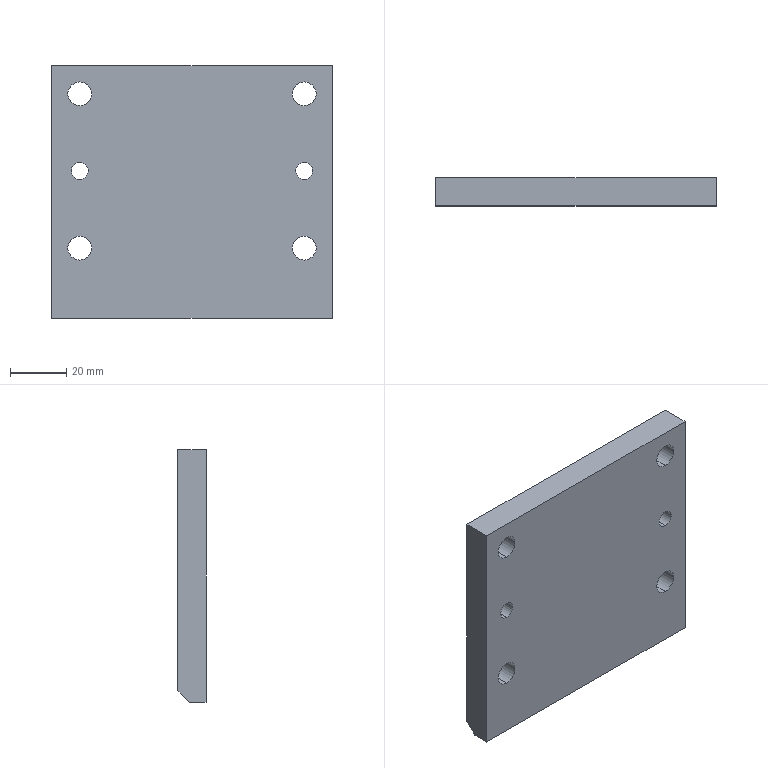Part | STEP file | X77-02101 | 1 solid | 19 faces | box 100 x 10 x 90 mm | volume 86365 mm3 | cylinder 12 | plane 7 | commonest cylinder face diameters 8.5 x8 6 x4
STEP:
#1=CARTESIAN_POINT('',(30.,-123.,55.5));
#2=VERTEX_POINT('',#1);
#3=CARTESIAN_POINT('',(30.,-123.,49.5));
#4=VERTEX_POINT('',#3);
#5=CARTESIAN_POINT('',(30.,-123.,52.5));
#6=DIRECTION('',(0.,-1.,0.));
#7=DIRECTION('',(0.,0.,1.));
#8=AXIS2_PLACEMENT_3D('',#5,#6,#7);
#9=CIRCLE('',#8,3.);
#10=EDGE_CURVE('',#2,#4,#9,.T.);
#11=ORIENTED_EDGE('',*,*,#10,.T.);
#12=CARTESIAN_POINT('',(30.,-113.,49.5));
#13=VERTEX_POINT('',#12);
#14=CARTESIAN_POINT('',(30.,-125.,49.5));
#15=DIRECTION('',(0.,1.,0.));
#16=VECTOR('',#15,1000.);
#17=LINE('',#14,#16);
#18=EDGE_CURVE('',#4,#13,#17,.T.);
#19=ORIENTED_EDGE('',*,*,#18,.T.);
#20=CARTESIAN_POINT('',(30.,-113.,55.5));
#21=VERTEX_POINT('',#20);
#22=CARTESIAN_POINT('',(30.,-113.,52.5));
#23=DIRECTION('',(0.,1.,0.));
#24=DIRECTION('',(0.,0.,1.));
#25=AXIS2_PLACEMENT_3D('',#22,#23,#24);
#26=CIRCLE('',#25,3.);
#27=EDGE_CURVE('',#13,#21,#26,.T.);
#28=ORIENTED_EDGE('',*,*,#27,.T.);
#29=CARTESIAN_POINT('',(30.,-125.,55.5));
#30=DIRECTION('',(0.,1.,0.));
#31=VECTOR('',#30,1000.);
#32=LINE('',#29,#31);
#33=EDGE_CURVE('',#2,#21,#32,.T.);
#34=ORIENTED_EDGE('',*,*,#33,.F.);
#35=EDGE_LOOP('',(#11,#19,#28,#34));
#36=FACE_OUTER_BOUND('',#35,.T.);
#37=CARTESIAN_POINT('',(30.,-125.,52.5));
#38=DIRECTION('',(0.,1.,0.));
#39=DIRECTION('',(0.,0.,1.));
#40=AXIS2_PLACEMENT_3D('',#37,#38,#39);
#41=CYLINDRICAL_SURFACE('',#40,3.);
#42=ADVANCED_FACE('',(#36),#41,.F.);
#43=CARTESIAN_POINT('',(-50.,-123.,55.5));
#44=VERTEX_POINT('',#43);
#45=CARTESIAN_POINT('',(-50.,-123.,49.5));
#46=VERTEX_POINT('',#45);
#47=CARTESIAN_POINT('',(-50.,-123.,52.5));
#48=DIRECTION('',(0.,-1.,0.));
#49=DIRECTION('',(0.,0.,1.));
#50=AXIS2_PLACEMENT_3D('',#47,#48,#49);
#51=CIRCLE('',#50,3.);
#52=EDGE_CURVE('',#44,#46,#51,.T.);
#53=ORIENTED_EDGE('',*,*,#52,.T.);
#54=CARTESIAN_POINT('',(-50.,-113.,49.5));
#55=VERTEX_POINT('',#54);
#56=CARTESIAN_POINT('',(-50.,-125.,49.5));
#57=DIRECTION('',(0.,1.,0.));
#58=VECTOR('',#57,1000.);
#59=LINE('',#56,#58);
#60=EDGE_CURVE('',#46,#55,#59,.T.);
#61=ORIENTED_EDGE('',*,*,#60,.T.);
#62=CARTESIAN_POINT('',(-50.,-113.,55.5));
#63=VERTEX_POINT('',#62);
#64=CARTESIAN_POINT('',(-50.,-113.,52.5));
#65=DIRECTION('',(0.,1.,0.));
#66=DIRECTION('',(0.,0.,1.));
#67=AXIS2_PLACEMENT_3D('',#64,#65,#66);
#68=CIRCLE('',#67,3.);
#69=EDGE_CURVE('',#55,#63,#68,.T.);
#70=ORIENTED_EDGE('',*,*,#69,.T.);
#71=CARTESIAN_POINT('',(-50.,-125.,55.5));
#72=DIRECTION('',(0.,1.,0.));
#73=VECTOR('',#72,1000.);
#74=LINE('',#71,#73);
#75=EDGE_CURVE('',#44,#63,#74,.T.);
#76=ORIENTED_EDGE('',*,*,#75,.F.);
#77=EDGE_LOOP('',(#53,#61,#70,#76));
#78=FACE_OUTER_BOUND('',#77,.T.);
#79=CARTESIAN_POINT('',(-50.,-125.,52.5));
#80=DIRECTION('',(0.,1.,0.));
#81=DIRECTION('',(0.,0.,1.));
#82=AXIS2_PLACEMENT_3D('',#79,#80,#81);
#83=CYLINDRICAL_SURFACE('',#82,3.);
#84=ADVANCED_FACE('',(#78),#83,.F.);
#85=CARTESIAN_POINT('',(-50.,-123.,84.25));
#86=VERTEX_POINT('',#85);
#87=CARTESIAN_POINT('',(-50.,-123.,75.75));
#88=VERTEX_POINT('',#87);
#89=CARTESIAN_POINT('',(-50.,-123.,80.));
#90=DIRECTION('',(0.,-1.,0.));
#91=DIRECTION('',(0.,0.,1.));
#92=AXIS2_PLACEMENT_3D('',#89,#90,#91);
#93=CIRCLE('',#92,4.25);
#94=EDGE_CURVE('',#86,#88,#93,.T.);
#95=ORIENTED_EDGE('',*,*,#94,.T.);
#96=CARTESIAN_POINT('',(-50.,-113.,75.75));
#97=VERTEX_POINT('',#96);
#98=CARTESIAN_POINT('',(-50.,-113.,75.75));
#99=DIRECTION('',(0.,1.,0.));
#100=VECTOR('',#99,1000.);
#101=LINE('',#98,#100);
#102=EDGE_CURVE('',#88,#97,#101,.T.);
#103=ORIENTED_EDGE('',*,*,#102,.T.);
#104=CARTESIAN_POINT('',(-50.,-113.,84.25));
#105=VERTEX_POINT('',#104);
#106=CARTESIAN_POINT('',(-50.,-113.,80.));
#107=DIRECTION('',(0.,1.,0.));
#108=DIRECTION('',(0.,0.,1.));
#109=AXIS2_PLACEMENT_3D('',#106,#107,#108);
#110=CIRCLE('',#109,4.25);
#111=EDGE_CURVE('',#97,#105,#110,.T.);
#112=ORIENTED_EDGE('',*,*,#111,.T.);
#113=CARTESIAN_POINT('',(-50.,-113.,84.25));
#114=DIRECTION('',(0.,1.,0.));
#115=VECTOR('',#114,1000.);
#116=LINE('',#113,#115);
#117=EDGE_CURVE('',#86,#105,#116,.T.);
#118=ORIENTED_EDGE('',*,*,#117,.F.);
#119=EDGE_LOOP('',(#95,#103,#112,#118));
#120=FACE_OUTER_BOUND('',#119,.T.);
#121=CARTESIAN_POINT('',(-50.,-113.,80.));
#122=DIRECTION('',(0.,1.,0.));
#123=DIRECTION('',(0.,0.,1.));
#124=AXIS2_PLACEMENT_3D('',#121,#122,#123);
#125=CYLINDRICAL_SURFACE('',#124,4.25);
#126=ADVANCED_FACE('',(#120),#125,.F.);
#127=CARTESIAN_POINT('',(-50.,-123.,29.25));
#128=VERTEX_POINT('',#127);
#129=CARTESIAN_POINT('',(-50.,-123.,20.75));
#130=VERTEX_POINT('',#129);
#131=CARTESIAN_POINT('',(-50.,-123.,25.));
#132=DIRECTION('',(0.,-1.,0.));
#133=DIRECTION('',(0.,0.,1.));
#134=AXIS2_PLACEMENT_3D('',#131,#132,#133);
#135=CIRCLE('',#134,4.25);
#136=EDGE_CURVE('',#128,#130,#135,.T.);
#137=ORIENTED_EDGE('',*,*,#136,.T.);
#138=CARTESIAN_POINT('',(-50.,-113.,20.75));
#139=VERTEX_POINT('',#138);
#140=CARTESIAN_POINT('',(-50.,-113.,20.75));
#141=DIRECTION('',(0.,1.,0.));
#142=VECTOR('',#141,1000.);
#143=LINE('',#140,#142);
#144=EDGE_CURVE('',#130,#139,#143,.T.);
#145=ORIENTED_EDGE('',*,*,#144,.T.);
#146=CARTESIAN_POINT('',(-50.,-113.,29.25));
#147=VERTEX_POINT('',#146);
#148=CARTESIAN_POINT('',(-50.,-113.,25.));
#149=DIRECTION('',(0.,1.,0.));
#150=DIRECTION('',(0.,0.,1.));
#151=AXIS2_PLACEMENT_3D('',#148,#149,#150);
#152=CIRCLE('',#151,4.25);
#153=EDGE_CURVE('',#139,#147,#152,.T.);
#154=ORIENTED_EDGE('',*,*,#153,.T.);
#155=CARTESIAN_POINT('',(-50.,-113.,29.25));
#156=DIRECTION('',(0.,1.,0.));
#157=VECTOR('',#156,1000.);
#158=LINE('',#155,#157);
#159=EDGE_CURVE('',#128,#147,#158,.T.);
#160=ORIENTED_EDGE('',*,*,#159,.F.);
#161=EDGE_LOOP('',(#137,#145,#154,#160));
#162=FACE_OUTER_BOUND('',#161,.T.);
#163=CARTESIAN_POINT('',(-50.,-113.,25.));
#164=DIRECTION('',(0.,1.,0.));
#165=DIRECTION('',(0.,0.,1.));
#166=AXIS2_PLACEMENT_3D('',#163,#164,#165);
#167=CYLINDRICAL_SURFACE('',#166,4.25);
#168=ADVANCED_FACE('',(#162),#167,.F.);
#169=CARTESIAN_POINT('',(30.,-123.,29.25));
#170=VERTEX_POINT('',#169);
#171=CARTESIAN_POINT('',(30.,-123.,20.75));
#172=VERTEX_POINT('',#171);
#173=CARTESIAN_POINT('',(30.,-123.,25.));
#174=DIRECTION('',(0.,-1.,0.));
#175=DIRECTION('',(0.,0.,1.));
#176=AXIS2_PLACEMENT_3D('',#173,#174,#175);
#177=CIRCLE('',#176,4.25);
#178=EDGE_CURVE('',#170,#172,#177,.T.);
#179=ORIENTED_EDGE('',*,*,#178,.T.);
#180=CARTESIAN_POINT('',(30.,-113.,20.75));
#181=VERTEX_POINT('',#180);
#182=CARTESIAN_POINT('',(30.,-113.,20.75));
#183=DIRECTION('',(0.,1.,0.));
#184=VECTOR('',#183,1000.);
#185=LINE('',#182,#184);
#186=EDGE_CURVE('',#172,#181,#185,.T.);
#187=ORIENTED_EDGE('',*,*,#186,.T.);
#188=CARTESIAN_POINT('',(30.,-113.,29.25));
#189=VERTEX_POINT('',#188);
#190=CARTESIAN_POINT('',(30.,-113.,25.));
#191=DIRECTION('',(0.,1.,0.));
#192=DIRECTION('',(0.,0.,1.));
#193=AXIS2_PLACEMENT_3D('',#190,#191,#192);
#194=CIRCLE('',#193,4.25);
#195=EDGE_CURVE('',#181,#189,#194,.T.);
#196=ORIENTED_EDGE('',*,*,#195,.T.);
#197=CARTESIAN_POINT('',(30.,-113.,29.25));
#198=DIRECTION('',(0.,1.,0.));
#199=VECTOR('',#198,1000.);
#200=LINE('',#197,#199);
#201=EDGE_CURVE('',#170,#189,#200,.T.);
#202=ORIENTED_EDGE('',*,*,#201,.F.);
#203=EDGE_LOOP('',(#179,#187,#196,#202));
#204=FACE_OUTER_BOUND('',#203,.T.);
#205=CARTESIAN_POINT('',(30.,-113.,25.));
#206=DIRECTION('',(0.,1.,0.));
#207=DIRECTION('',(0.,0.,1.));
#208=AXIS2_PLACEMENT_3D('',#205,#206,#207);
#209=CYLINDRICAL_SURFACE('',#208,4.25);
#210=ADVANCED_FACE('',(#204),#209,.F.);
#211=CARTESIAN_POINT('',(30.,-123.,84.25));
#212=VERTEX_POINT('',#211);
#213=CARTESIAN_POINT('',(30.,-123.,75.75));
#214=VERTEX_POINT('',#213);
#215=CARTESIAN_POINT('',(30.,-123.,80.));
#216=DIRECTION('',(0.,-1.,0.));
#217=DIRECTION('',(0.,0.,1.));
#218=AXIS2_PLACEMENT_3D('',#215,#216,#217);
#219=CIRCLE('',#218,4.25);
#220=EDGE_CURVE('',#212,#214,#219,.T.);
#221=ORIENTED_EDGE('',*,*,#220,.T.);
#222=CARTESIAN_POINT('',(30.,-113.,75.75));
#223=VERTEX_POINT('',#222);
#224=CARTESIAN_POINT('',(30.,-113.,75.75));
#225=DIRECTION('',(0.,1.,0.));
#226=VECTOR('',#225,1000.);
#227=LINE('',#224,#226);
#228=EDGE_CURVE('',#214,#223,#227,.T.);
#229=ORIENTED_EDGE('',*,*,#228,.T.);
#230=CARTESIAN_POINT('',(30.,-113.,84.25));
#231=VERTEX_POINT('',#230);
#232=CARTESIAN_POINT('',(30.,-113.,80.));
#233=DIRECTION('',(0.,1.,0.));
#234=DIRECTION('',(0.,0.,1.));
#235=AXIS2_PLACEMENT_3D('',#232,#233,#234);
#236=CIRCLE('',#235,4.25);
#237=EDGE_CURVE('',#223,#231,#236,.T.);
#238=ORIENTED_EDGE('',*,*,#237,.T.);
#239=CARTESIAN_POINT('',(30.,-113.,84.25));
#240=DIRECTION('',(0.,1.,0.));
#241=VECTOR('',#240,1000.);
#242=LINE('',#239,#241);
#243=EDGE_CURVE('',#212,#231,#242,.T.);
#244=ORIENTED_EDGE('',*,*,#243,.F.);
#245=EDGE_LOOP('',(#221,#229,#238,#244));
#246=FACE_OUTER_BOUND('',#245,.T.);
#247=CARTESIAN_POINT('',(30.,-113.,80.));
#248=DIRECTION('',(0.,1.,0.));
#249=DIRECTION('',(0.,0.,1.));
#250=AXIS2_PLACEMENT_3D('',#247,#248,#249);
#251=CYLINDRICAL_SURFACE('',#250,4.25);
#252=ADVANCED_FACE('',(#246),#251,.F.);
#253=CARTESIAN_POINT('',(-60.,-117.,0.));
#254=VERTEX_POINT('',#253);
#255=CARTESIAN_POINT('',(-60.,-123.,0.));
#256=VERTEX_POINT('',#255);
#257=CARTESIAN_POINT('',(-60.,-125.,0.));
#258=DIRECTION('',(0.,-1.,0.));
#259=VECTOR('',#258,1000.);
#260=LINE('',#257,#259);
#261=EDGE_CURVE('',#254,#256,#260,.T.);
#262=ORIENTED_EDGE('',*,*,#261,.T.);
#263=CARTESIAN_POINT('',(-60.,-123.,90.));
#264=VERTEX_POINT('',#263);
#265=CARTESIAN_POINT('',(-60.,-123.,0.));
#266=DIRECTION('',(0.,0.,-1.));
#267=VECTOR('',#266,1000.);
#268=LINE('',#265,#267);
#269=EDGE_CURVE('',#264,#256,#268,.T.);
#270=ORIENTED_EDGE('',*,*,#269,.F.);
#271=CARTESIAN_POINT('',(-60.,-113.,90.));
#272=VERTEX_POINT('',#271);
#273=CARTESIAN_POINT('',(-60.,-125.,90.));
#274=DIRECTION('',(0.,-1.,0.));
#275=VECTOR('',#274,1000.);
#276=LINE('',#273,#275);
#277=EDGE_CURVE('',#272,#264,#276,.T.);
#278=ORIENTED_EDGE('',*,*,#277,.F.);
#279=CARTESIAN_POINT('',(-60.,-113.,4.));
#280=VERTEX_POINT('',#279);
#281=CARTESIAN_POINT('',(-60.,-113.,90.));
#282=DIRECTION('',(0.,0.,-1.));
#283=VECTOR('',#282,1000.);
#284=LINE('',#281,#283);
#285=EDGE_CURVE('',#272,#280,#284,.T.);
#286=ORIENTED_EDGE('',*,*,#285,.T.);
#287=CARTESIAN_POINT('',(-60.,-113.,4.));
#288=DIRECTION('',(0.,-0.7071,-0.7071));
#289=VECTOR('',#288,1000.);
#290=LINE('',#287,#289);
#291=EDGE_CURVE('',#280,#254,#290,.T.);
#292=ORIENTED_EDGE('',*,*,#291,.T.);
#293=EDGE_LOOP('',(#262,#270,#278,#286,#292));
#294=FACE_OUTER_BOUND('',#293,.T.);
#295=CARTESIAN_POINT('',(-60.,-125.,90.));
#296=DIRECTION('',(1.,0.,0.));
#297=DIRECTION('',(0.,0.,-1.));
#298=AXIS2_PLACEMENT_3D('',#295,#296,#297);
#299=PLANE('',#298);
#300=ADVANCED_FACE('',(#294),#299,.F.);
#301=CARTESIAN_POINT('',(40.,-123.,90.));
#302=VERTEX_POINT('',#301);
#303=CARTESIAN_POINT('',(40.,-113.,90.));
#304=VERTEX_POINT('',#303);
#305=CARTESIAN_POINT('',(40.,-125.,90.));
#306=DIRECTION('',(0.,1.,0.));
#307=VECTOR('',#306,1000.);
#308=LINE('',#305,#307);
#309=EDGE_CURVE('',#302,#304,#308,.T.);
#310=ORIENTED_EDGE('',*,*,#309,.F.);
#311=CARTESIAN_POINT('',(40.,-123.,0.));
#312=VERTEX_POINT('',#311);
#313=CARTESIAN_POINT('',(40.,-123.,0.));
#314=DIRECTION('',(0.,0.,-1.));
#315=VECTOR('',#314,1000.);
#316=LINE('',#313,#315);
#317=EDGE_CURVE('',#302,#312,#316,.T.);
#318=ORIENTED_EDGE('',*,*,#317,.T.);
#319=CARTESIAN_POINT('',(40.,-117.,0.));
#320=VERTEX_POINT('',#319);
#321=CARTESIAN_POINT('',(40.,-125.,0.));
#322=DIRECTION('',(0.,1.,0.));
#323=VECTOR('',#322,1000.);
#324=LINE('',#321,#323);
#325=EDGE_CURVE('',#312,#320,#324,.T.);
#326=ORIENTED_EDGE('',*,*,#325,.T.);
#327=CARTESIAN_POINT('',(40.,-113.,4.));
#328=VERTEX_POINT('',#327);
#329=CARTESIAN_POINT('',(40.,-113.,4.));
#330=DIRECTION('',(0.,0.7071,0.7071));
#331=VECTOR('',#330,1000.);
#332=LINE('',#329,#331);
#333=EDGE_CURVE('',#320,#328,#332,.T.);
#334=ORIENTED_EDGE('',*,*,#333,.T.);
#335=CARTESIAN_POINT('',(40.,-113.,90.));
#336=DIRECTION('',(0.,0.,-1.));
#337=VECTOR('',#336,1000.);
#338=LINE('',#335,#337);
#339=EDGE_CURVE('',#304,#328,#338,.T.);
#340=ORIENTED_EDGE('',*,*,#339,.F.);
#341=EDGE_LOOP('',(#310,#318,#326,#334,#340));
#342=FACE_OUTER_BOUND('',#341,.T.);
#343=CARTESIAN_POINT('',(40.,-125.,90.));
#344=DIRECTION('',(-1.,0.,0.));
#345=DIRECTION('',(0.,0.,1.));
#346=AXIS2_PLACEMENT_3D('',#343,#344,#345);
#347=PLANE('',#346);
#348=ADVANCED_FACE('',(#342),#347,.F.);
#349=CARTESIAN_POINT('',(30.,-113.,52.5));
#350=DIRECTION('',(0.,1.,0.));
#351=DIRECTION('',(0.,0.,1.));
#352=AXIS2_PLACEMENT_3D('',#349,#350,#351);
#353=CIRCLE('',#352,3.);
#354=EDGE_CURVE('',#21,#13,#353,.T.);
#355=ORIENTED_EDGE('',*,*,#354,.F.);
#356=ORIENTED_EDGE('',*,*,#27,.F.);
#357=EDGE_LOOP('',(#355,#356));
#358=FACE_BOUND('',#357,.T.);
#359=CARTESIAN_POINT('',(-50.,-113.,52.5));
#360=DIRECTION('',(0.,1.,0.));
#361=DIRECTION('',(0.,0.,1.));
#362=AXIS2_PLACEMENT_3D('',#359,#360,#361);
#363=CIRCLE('',#362,3.);
#364=EDGE_CURVE('',#63,#55,#363,.T.);
#365=ORIENTED_EDGE('',*,*,#364,.F.);
#366=ORIENTED_EDGE('',*,*,#69,.F.);
#367=EDGE_LOOP('',(#365,#366));
#368=FACE_BOUND('',#367,.T.);
#369=CARTESIAN_POINT('',(-50.,-113.,80.));
#370=DIRECTION('',(0.,1.,0.));
#371=DIRECTION('',(0.,0.,1.));
#372=AXIS2_PLACEMENT_3D('',#369,#370,#371);
#373=CIRCLE('',#372,4.25);
#374=EDGE_CURVE('',#105,#97,#373,.T.);
#375=ORIENTED_EDGE('',*,*,#374,.F.);
#376=ORIENTED_EDGE('',*,*,#111,.F.);
#377=EDGE_LOOP('',(#375,#376));
#378=FACE_BOUND('',#377,.T.);
#379=CARTESIAN_POINT('',(-50.,-113.,25.));
#380=DIRECTION('',(0.,1.,0.));
#381=DIRECTION('',(0.,0.,1.));
#382=AXIS2_PLACEMENT_3D('',#379,#380,#381);
#383=CIRCLE('',#382,4.25);
#384=EDGE_CURVE('',#147,#139,#383,.T.);
#385=ORIENTED_EDGE('',*,*,#384,.F.);
#386=ORIENTED_EDGE('',*,*,#153,.F.);
#387=EDGE_LOOP('',(#385,#386));
#388=FACE_BOUND('',#387,.T.);
#389=CARTESIAN_POINT('',(30.,-113.,25.));
#390=DIRECTION('',(0.,1.,0.));
#391=DIRECTION('',(0.,0.,1.));
#392=AXIS2_PLACEMENT_3D('',#389,#390,#391);
#393=CIRCLE('',#392,4.25);
#394=EDGE_CURVE('',#189,#181,#393,.T.);
#395=ORIENTED_EDGE('',*,*,#394,.F.);
#396=ORIENTED_EDGE('',*,*,#195,.F.);
#397=EDGE_LOOP('',(#395,#396));
#398=FACE_BOUND('',#397,.T.);
#399=CARTESIAN_POINT('',(30.,-113.,80.));
#400=DIRECTION('',(0.,1.,0.));
#401=DIRECTION('',(0.,0.,1.));
#402=AXIS2_PLACEMENT_3D('',#399,#400,#401);
#403=CIRCLE('',#402,4.25);
#404=EDGE_CURVE('',#231,#223,#403,.T.);
#405=ORIENTED_EDGE('',*,*,#404,.F.);
#406=ORIENTED_EDGE('',*,*,#237,.F.);
#407=EDGE_LOOP('',(#405,#406));
#408=FACE_BOUND('',#407,.T.);
#409=ORIENTED_EDGE('',*,*,#339,.T.);
#410=CARTESIAN_POINT('',(-60.,-113.,4.));
#411=DIRECTION('',(-1.,0.,0.));
#412=VECTOR('',#411,1000.);
#413=LINE('',#410,#412);
#414=EDGE_CURVE('',#328,#280,#413,.T.);
#415=ORIENTED_EDGE('',*,*,#414,.T.);
#416=ORIENTED_EDGE('',*,*,#285,.F.);
#417=CARTESIAN_POINT('',(-60.,-113.,90.));
#418=DIRECTION('',(-1.,0.,0.));
#419=VECTOR('',#418,1000.);
#420=LINE('',#417,#419);
#421=EDGE_CURVE('',#304,#272,#420,.T.);
#422=ORIENTED_EDGE('',*,*,#421,.F.);
#423=EDGE_LOOP('',(#409,#415,#416,#422));
#424=FACE_OUTER_BOUND('',#423,.T.);
#425=CARTESIAN_POINT('',(-60.,-113.,90.));
#426=DIRECTION('',(0.,-1.,0.));
#427=DIRECTION('',(0.,0.,-1.));
#428=AXIS2_PLACEMENT_3D('',#425,#426,#427);
#429=PLANE('',#428);
#430=ADVANCED_FACE('',(#358,#368,#378,#388,#398,#408,#424),#429,.F.);
#431=ORIENTED_EDGE('',*,*,#277,.T.);
#432=CARTESIAN_POINT('',(40.,-123.,90.));
#433=DIRECTION('',(-1.,0.,0.));
#434=VECTOR('',#433,1000.);
#435=LINE('',#432,#434);
#436=EDGE_CURVE('',#302,#264,#435,.T.);
#437=ORIENTED_EDGE('',*,*,#436,.F.);
#438=ORIENTED_EDGE('',*,*,#309,.T.);
#439=ORIENTED_EDGE('',*,*,#421,.T.);
#440=EDGE_LOOP('',(#431,#437,#438,#439));
#441=FACE_OUTER_BOUND('',#440,.T.);
#442=CARTESIAN_POINT('',(-60.,-113.,90.));
#443=DIRECTION('',(0.,0.,-1.));
#444=DIRECTION('',(-1.,0.,0.));
#445=AXIS2_PLACEMENT_3D('',#442,#443,#444);
#446=PLANE('',#445);
#447=ADVANCED_FACE('',(#441),#446,.F.);
#448=CARTESIAN_POINT('',(40.,-123.,0.));
#449=DIRECTION('',(-1.,0.,0.));
#450=VECTOR('',#449,1000.);
#451=LINE('',#448,#450);
#452=EDGE_CURVE('',#312,#256,#451,.T.);
#453=ORIENTED_EDGE('',*,*,#452,.T.);
#454=ORIENTED_EDGE('',*,*,#261,.F.);
#455=CARTESIAN_POINT('',(40.,-117.,0.));
#456=DIRECTION('',(1.,0.,0.));
#457=VECTOR('',#456,1000.);
#458=LINE('',#455,#457);
#459=EDGE_CURVE('',#254,#320,#458,.T.);
#460=ORIENTED_EDGE('',*,*,#459,.T.);
#461=ORIENTED_EDGE('',*,*,#325,.F.);
#462=EDGE_LOOP('',(#453,#454,#460,#461));
#463=FACE_OUTER_BOUND('',#462,.T.);
#464=CARTESIAN_POINT('',(-60.,-113.,0.));
#465=DIRECTION('',(0.,0.,-1.));
#466=DIRECTION('',(-1.,0.,0.));
#467=AXIS2_PLACEMENT_3D('',#464,#465,#466);
#468=PLANE('',#467);
#469=ADVANCED_FACE('',(#463),#468,.T.);
#470=ORIENTED_EDGE('',*,*,#228,.F.);
#471=CARTESIAN_POINT('',(30.,-123.,80.));
#472=DIRECTION('',(0.,-1.,0.));
#473=DIRECTION('',(0.,0.,1.));
#474=AXIS2_PLACEMENT_3D('',#471,#472,#473);
#475=CIRCLE('',#474,4.25);
#476=EDGE_CURVE('',#214,#212,#475,.T.);
#477=ORIENTED_EDGE('',*,*,#476,.T.);
#478=ORIENTED_EDGE('',*,*,#243,.T.);
#479=ORIENTED_EDGE('',*,*,#404,.T.);
#480=EDGE_LOOP('',(#470,#477,#478,#479));
#481=FACE_OUTER_BOUND('',#480,.T.);
#482=CARTESIAN_POINT('',(30.,-113.,80.));
#483=DIRECTION('',(0.,1.,0.));
#484=DIRECTION('',(0.,0.,1.));
#485=AXIS2_PLACEMENT_3D('',#482,#483,#484);
#486=CYLINDRICAL_SURFACE('',#485,4.25);
#487=ADVANCED_FACE('',(#481),#486,.F.);
#488=ORIENTED_EDGE('',*,*,#186,.F.);
#489=CARTESIAN_POINT('',(30.,-123.,25.));
#490=DIRECTION('',(0.,-1.,0.));
#491=DIRECTION('',(0.,0.,1.));
#492=AXIS2_PLACEMENT_3D('',#489,#490,#491);
#493=CIRCLE('',#492,4.25);
#494=EDGE_CURVE('',#172,#170,#493,.T.);
#495=ORIENTED_EDGE('',*,*,#494,.T.);
#496=ORIENTED_EDGE('',*,*,#201,.T.);
#497=ORIENTED_EDGE('',*,*,#394,.T.);
#498=EDGE_LOOP('',(#488,#495,#496,#497));
#499=FACE_OUTER_BOUND('',#498,.T.);
#500=CARTESIAN_POINT('',(30.,-113.,25.));
#501=DIRECTION('',(0.,1.,0.));
#502=DIRECTION('',(0.,0.,1.));
#503=AXIS2_PLACEMENT_3D('',#500,#501,#502);
#504=CYLINDRICAL_SURFACE('',#503,4.25);
#505=ADVANCED_FACE('',(#499),#504,.F.);
#506=ORIENTED_EDGE('',*,*,#144,.F.);
#507=CARTESIAN_POINT('',(-50.,-123.,25.));
#508=DIRECTION('',(0.,-1.,0.));
#509=DIRECTION('',(0.,0.,1.));
#510=AXIS2_PLACEMENT_3D('',#507,#508,#509);
#511=CIRCLE('',#510,4.25);
#512=EDGE_CURVE('',#130,#128,#511,.T.);
#513=ORIENTED_EDGE('',*,*,#512,.T.);
#514=ORIENTED_EDGE('',*,*,#159,.T.);
#515=ORIENTED_EDGE('',*,*,#384,.T.);
#516=EDGE_LOOP('',(#506,#513,#514,#515));
#517=FACE_OUTER_BOUND('',#516,.T.);
#518=CARTESIAN_POINT('',(-50.,-113.,25.));
#519=DIRECTION('',(0.,1.,0.));
#520=DIRECTION('',(0.,0.,1.));
#521=AXIS2_PLACEMENT_3D('',#518,#519,#520);
#522=CYLINDRICAL_SURFACE('',#521,4.25);
#523=ADVANCED_FACE('',(#517),#522,.F.);
#524=ORIENTED_EDGE('',*,*,#102,.F.);
#525=CARTESIAN_POINT('',(-50.,-123.,80.));
#526=DIRECTION('',(0.,-1.,0.));
#527=DIRECTION('',(0.,0.,1.));
#528=AXIS2_PLACEMENT_3D('',#525,#526,#527);
#529=CIRCLE('',#528,4.25);
#530=EDGE_CURVE('',#88,#86,#529,.T.);
#531=ORIENTED_EDGE('',*,*,#530,.T.);
#532=ORIENTED_EDGE('',*,*,#117,.T.);
#533=ORIENTED_EDGE('',*,*,#374,.T.);
#534=EDGE_LOOP('',(#524,#531,#532,#533));
#535=FACE_OUTER_BOUND('',#534,.T.);
#536=CARTESIAN_POINT('',(-50.,-113.,80.));
#537=DIRECTION('',(0.,1.,0.));
#538=DIRECTION('',(0.,0.,1.));
#539=AXIS2_PLACEMENT_3D('',#536,#537,#538);
#540=CYLINDRICAL_SURFACE('',#539,4.25);
#541=ADVANCED_FACE('',(#535),#540,.F.);
#542=ORIENTED_EDGE('',*,*,#60,.F.);
#543=CARTESIAN_POINT('',(-50.,-123.,52.5));
#544=DIRECTION('',(0.,-1.,0.));
#545=DIRECTION('',(0.,0.,1.));
#546=AXIS2_PLACEMENT_3D('',#543,#544,#545);
#547=CIRCLE('',#546,3.);
#548=EDGE_CURVE('',#46,#44,#547,.T.);
#549=ORIENTED_EDGE('',*,*,#548,.T.);
#550=ORIENTED_EDGE('',*,*,#75,.T.);
#551=ORIENTED_EDGE('',*,*,#364,.T.);
#552=EDGE_LOOP('',(#542,#549,#550,#551));
#553=FACE_OUTER_BOUND('',#552,.T.);
#554=CARTESIAN_POINT('',(-50.,-125.,52.5));
#555=DIRECTION('',(0.,1.,0.));
#556=DIRECTION('',(0.,0.,1.));
#557=AXIS2_PLACEMENT_3D('',#554,#555,#556);
#558=CYLINDRICAL_SURFACE('',#557,3.);
#559=ADVANCED_FACE('',(#553),#558,.F.);
#560=ORIENTED_EDGE('',*,*,#18,.F.);
#561=CARTESIAN_POINT('',(30.,-123.,52.5));
#562=DIRECTION('',(0.,-1.,0.));
#563=DIRECTION('',(0.,0.,1.));
#564=AXIS2_PLACEMENT_3D('',#561,#562,#563);
#565=CIRCLE('',#564,3.);
#566=EDGE_CURVE('',#4,#2,#565,.T.);
#567=ORIENTED_EDGE('',*,*,#566,.T.);
#568=ORIENTED_EDGE('',*,*,#33,.T.);
#569=ORIENTED_EDGE('',*,*,#354,.T.);
#570=EDGE_LOOP('',(#560,#567,#568,#569));
#571=FACE_OUTER_BOUND('',#570,.T.);
#572=CARTESIAN_POINT('',(30.,-125.,52.5));
#573=DIRECTION('',(0.,1.,0.));
#574=DIRECTION('',(0.,0.,1.));
#575=AXIS2_PLACEMENT_3D('',#572,#573,#574);
#576=CYLINDRICAL_SURFACE('',#575,3.);
#577=ADVANCED_FACE('',(#571),#576,.F.);
#578=ORIENTED_EDGE('',*,*,#333,.F.);
#579=ORIENTED_EDGE('',*,*,#459,.F.);
#580=ORIENTED_EDGE('',*,*,#291,.F.);
#581=ORIENTED_EDGE('',*,*,#414,.F.);
#582=EDGE_LOOP('',(#578,#579,#580,#581));
#583=FACE_OUTER_BOUND('',#582,.T.);
#584=CARTESIAN_POINT('',(-60.,-113.,4.));
#585=DIRECTION('',(0.,0.7071,-0.7071));
#586=DIRECTION('',(0.,0.7071,0.7071));
#587=AXIS2_PLACEMENT_3D('',#584,#585,#586);
#588=PLANE('',#587);
#589=ADVANCED_FACE('',(#583),#588,.T.);
#590=ORIENTED_EDGE('',*,*,#178,.F.);
#591=ORIENTED_EDGE('',*,*,#494,.F.);
#592=EDGE_LOOP('',(#590,#591));
#593=FACE_BOUND('',#592,.T.);
#594=ORIENTED_EDGE('',*,*,#94,.F.);
#595=ORIENTED_EDGE('',*,*,#530,.F.);
#596=EDGE_LOOP('',(#594,#595));
#597=FACE_BOUND('',#596,.T.);
#598=ORIENTED_EDGE('',*,*,#10,.F.);
#599=ORIENTED_EDGE('',*,*,#566,.F.);
#600=EDGE_LOOP('',(#598,#599));
#601=FACE_BOUND('',#600,.T.);
#602=ORIENTED_EDGE('',*,*,#269,.T.);
#603=ORIENTED_EDGE('',*,*,#452,.F.);
#604=ORIENTED_EDGE('',*,*,#317,.F.);
#605=ORIENTED_EDGE('',*,*,#436,.T.);
#606=EDGE_LOOP('',(#602,#603,#604,#605));
#607=FACE_OUTER_BOUND('',#606,.T.);
#608=ORIENTED_EDGE('',*,*,#52,.F.);
#609=ORIENTED_EDGE('',*,*,#548,.F.);
#610=EDGE_LOOP('',(#608,#609));
#611=FACE_BOUND('',#610,.T.);
#612=ORIENTED_EDGE('',*,*,#136,.F.);
#613=ORIENTED_EDGE('',*,*,#512,.F.);
#614=EDGE_LOOP('',(#612,#613));
#615=FACE_BOUND('',#614,.T.);
#616=ORIENTED_EDGE('',*,*,#220,.F.);
#617=ORIENTED_EDGE('',*,*,#476,.F.);
#618=EDGE_LOOP('',(#616,#617));
#619=FACE_BOUND('',#618,.T.);
#620=CARTESIAN_POINT('',(40.,-123.,0.));
#621=DIRECTION('',(0.,1.,0.));
#622=DIRECTION('',(0.,0.,1.));
#623=AXIS2_PLACEMENT_3D('',#620,#621,#622);
#624=PLANE('',#623);
#625=ADVANCED_FACE('',(#593,#597,#601,#607,#611,#615,#619),#624,.F.);
#626=CLOSED_SHELL('',(#42,#84,#126,#168,#210,#252,#300,#348,#430,#447,#469,#487,#505,#523,#541,#559,#577,#589,#625));
#627=MANIFOLD_SOLID_BREP('',#626);
#628=CARTESIAN_POINT('',(0.,0.,0.));
#629=DIRECTION('',(0.,0.,1.));
#630=DIRECTION('',(1.,0.,0.));
#631=AXIS2_PLACEMENT_3D('',#628,#629,#630);
#632=(LENGTH_UNIT()NAMED_UNIT(*)SI_UNIT(.MILLI.,.METRE.));
#633=UNCERTAINTY_MEASURE_WITH_UNIT(LENGTH_MEASURE(0.00001),#632,'','');
#634=(NAMED_UNIT(*)PLANE_ANGLE_UNIT()SI_UNIT($,.RADIAN.));
#635=(NAMED_UNIT(*)SI_UNIT($,.STERADIAN.)SOLID_ANGLE_UNIT());
#636=(GEOMETRIC_REPRESENTATION_CONTEXT(3)GLOBAL_UNCERTAINTY_ASSIGNED_CONTEXT((#633))GLOBAL_UNIT_ASSIGNED_CONTEXT((#632,#634,#635))REPRESENTATION_CONTEXT('',''));
#637=ADVANCED_BREP_SHAPE_REPRESENTATION('',(#627,#631),#636);